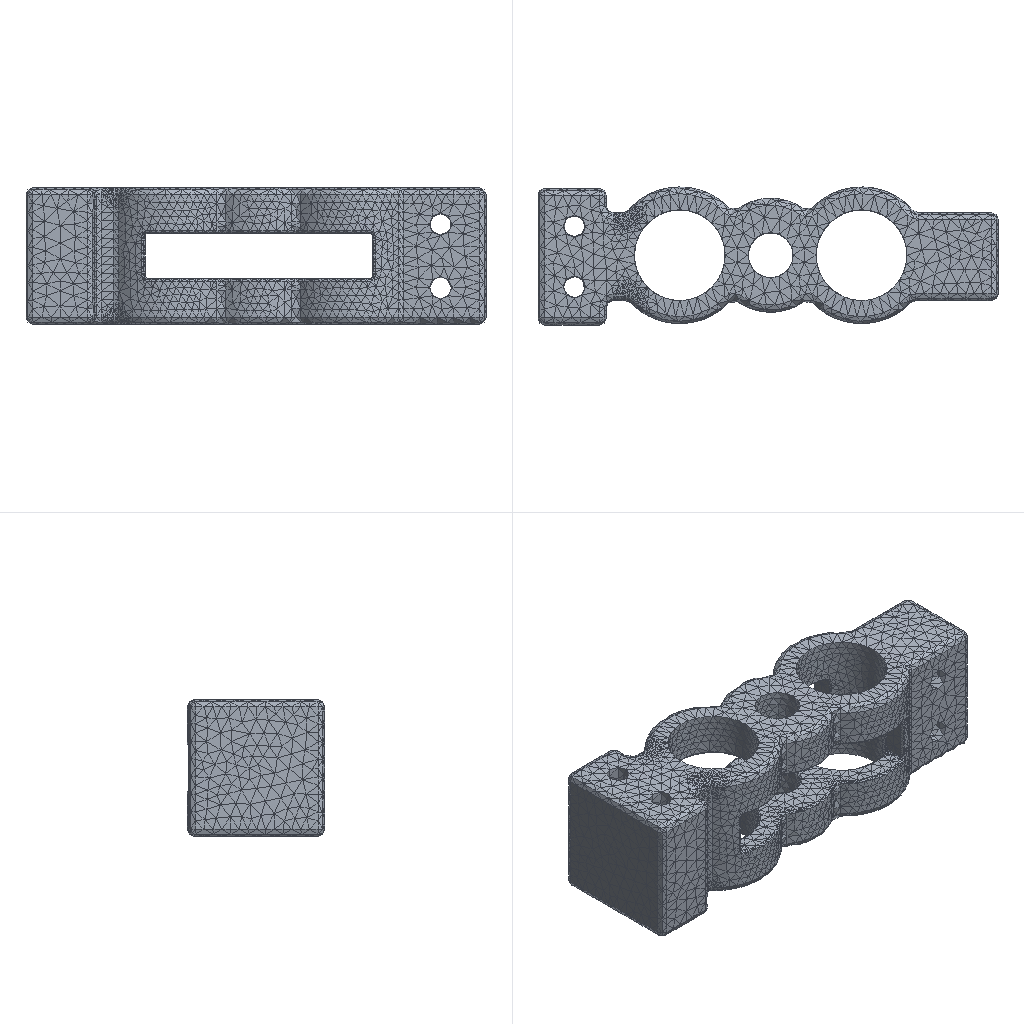Simulation study | ansys workbench
Set-up summary:
category,name,step,type,value,unit,region
solver,ansys_workbench
units,mm-N-s-tonne (MPa),,stated,"/units,MPA"
analysis,LS1,,static
load_step,LS1,LS1,static,nsubst=1; time=1
mesh,nodes,,,59608
mesh,elements,,,36199
element_type,SOLID187,,,35849
element_type,SURF154,,,350
material,Structural Steel,,E,200000,tonne s^-2 mm^-1
material,Structural Steel,,nu,0.3
material,Structural Steel,,density,7.85e-09,tonne mm^-3
material,Structural Steel,,conductivity,60.5,tonne mm s^-3 C^-1
material,Structural Steel,,specific_heat,4.34e+08,mm^2 s^-2 C^-1
material,Structural Steel,,cte,1.2e-05,C^-1
material,Structural Steel,,permeability,10000
material,Structural Steel,,resistivity,0.00017,ohm mm
load,Define Force Using Surface Effect Elements,LS1,surface-effect pres face 2,1.644,,SURF154 #2
bc,Fixed Supports,model,fixed,[dofs=ALL],,_FIXEDSU
named_set,_FIXEDSU,,node,576
Ansys APDL input file, long lists of numbers shortened:
/batch
/config,noeldb,1     ! force off writing results to database
*get,_wallstrt,active,,time,wall
! ANSYS input file written by Workbench version 2025 R2
! File used for geometry attach:
/title,wbnew--____ (A5)
! ****** Begin Custom Load Command Snippet ******
/COM, ACT Extensions:
/COM,     LSDYNA, 2025.2
/COM,/COM,     ANSYSMotion, 2025.2
/COM,
! ****** End   Custom Load Command Snippet ******
*DIM,_wb_ProjectScratch_dir,string,248
_wb_ProjectScratch_dir(1) = ''
*DIM,_wb_SolverFiles_dir,string,248
_wb_SolverFiles_dir(1) = ''
*DIM,_wb_userfiles_dir,string,248
_wb_userfiles_dir(1) = ''
/com,--- Data in consistent NMM units. See Solving Units in the help system for more information.
/units,MPA
/nopr
/wb,file,start              !  signify a WB generated input file
/prep7
! Turn off shape checking because checks already performed inside WB mesher.
! See help system for more information.
SHPP,OFF,,NOWARN
/nolist
etcon,set             ! allow ANSYS to choose best KEYOP's for 180x elements, resets any applicable keyopt to MAPDL defaults
/com,*********** Send User Defined Coordinate System(s) ***********
local,12,0,-71.019,0.4245,29.547,0.,0.,0.
local,13,0,-71.559,18.969,29.548,0.,0.,0.
local,14,0,-71.559,18.969,0.4524,0.,0.,0.
local,15,0,-71.019,0.4245,0.4529,0.,0.,0.
csys,0
/com,*********** Nodes for the whole assembly ***********
nblock,3,,65568
(1i9,3e20.9e3)
        1    -5.000000000E+01     1.000000000E+01     3.000000000E+01
! (59607 more lines like these left out)
-1
/wb,elem,start            !  set before creation of elements
/com,*********** Elements for Body 1 'Solid' ***********
et,1,187
MAT,1 $ TYPE,1 $ REAL,1 $ SECNUM,1 $ ESYS,0
eblock,11,COMPACT,,35849
(11i9)
        1     5950     9015     7975     8565    46217    57922    46214    46215    59404    57920
! (35848 more lines like these left out)
-1
secnum,1    ! reset the section ID to default
/wb,elem,end               !  done creating elements
toffst,273.15,      ! Temperature offset from absolute zero
/com,*********** Set Reference Temperature ***********
tref,22.
/wb,mat,start              !  starting to send materials
/com,*********** Send Materials ***********
Temperature = 'TEMP' ! Temperature
MP,DENS,1,7.85e-09,	! tonne mm^-3
MP,ALPX,1,1.2e-05,	! C^-1
MP,C,1,434000000,	! mm^2 s^-2 C^-1
MP,KXX,1,60.5,	! tonne mm s^-3 C^-1
MP,RSVX,1,0.00017,	! ohm mm
MP,EX,1,200000,	! tonne s^-2 mm^-1
MP,NUXY,1,0.3,
MP,MURX,1,10000,
/wb,mat,end                !  done sending materials
!************************* Model Summary ********************
!Solid,	结构钢,	matid,	1
!************************* End Model Summary ********************
! get the diagonal of the bounding box. Needed later for other things
*get,_xmin,node,,mnloc,x
*get,_ymin,node,,mnloc,y
*get,_zmin,node,,mnloc,z
*get,_xmax,node,,mxloc,x
*get,_ymax,node,,mxloc,y
*get,_zmax,node,,mxloc,z
_ASMDIAG=(_xmax-_xmin)*(_xmax-_xmin)+(_ymax-_ymin)*(_ymax-_ymin)+(_zmax-_zmin)*(_zmax-_zmin)
_ASMDIAG=SQRT(_ASMDIAG)
/wb,contact,start          !  starting to send contact
/wb,contact,end            !  done creating contacts
/golist
/wb,load,start             !  starting to send loads
/com,*********** Fixed Supports ***********
CMBLOCK,_FIXEDSU,NODE,      576
(8i10)
       287      -294       343      -350       514      -521       570      -577
! (71 more lines like these left out)
cmsel,s,_FIXEDSU
d,all,all
nsel,all
/com,*********** Define Force Using Surface Effect Elements ***********
local,16,0,0.,0.,0.,0.,0.,0.
csys,0
et,2,154
MAT,2 $ TYPE,2 $ REAL,2 $ SECNUM,2 $ ESYS,16
eblock,11,COMPACT,,350
(11i9)
    47220      791      790     4586     4586    14511    14513     4586    14519
! (349 more lines like these left out)
-1
secnum,1    ! reset the section ID to default
esel,s,type,,2
keyop,2,2,1         ! Apply load in local coordinate system
keyop,2,7,1         ! Use original area so load is constant in large deformation
esel,all
/gst,on,on
fini
*get,_numnode,node,0,count
*get,_numelem,elem,0,count
*get, _MAXELEMNUM, elem, 0, NUM, MAX
*get, _MAXNODENUM, node, 0, NUM, MAX
*get, _MAXELEMTYPE, etyp, 0, NUM, MAX
*get, _MAXREALCONST, rcon, 0, NUM, MAX
/go
/wb,load,end               !  done creating loads
/com,--- Number of total nodes = %_numnode%
/com,--- Number of contact elements = 350
/com,--- Number of spring elements = 0
/com,--- Number of bearing elements = 0
/com,--- Number of solid elements = 35849
/com,--- Number of condensed parts = 0
/com,--- Number of total elements = %_numelem%
*get,_wallbsol,active,,time,wall
/com,****************************************************************************
/com,*************************    SOLUTION       ********************************
/com,****************************************************************************
/solu
antype,0                   ! static analysis
_thickRatio=  1     ! Ratio of thick parts in the model
eqsl,pcg,1e-8,,,,,,1
cntr,print,1               ! print out contact info and also make no initial contact an error
cncheck,dmp		!	Enable program controlled contact splitting for distributed memory parallel run
dmpoption,emat,no             ! Don't combine emat file for DANSYS
dmpoption,esav,no             ! Don't combine esav file for DANSYS
nldiag,cont,iter           ! print out contact info each equilibrium iteration
rescontrol,,none                 ! Do not keep any restart files
/com,****************************************************
/com,******************* SOLVE FOR LS 1 OF 1 ****************
esel,s,type,,2
nsle
sfe,all,1,pres,1,0.
sfe,all,2,pres,1,1.644
sfe,all,3,pres,1,0.
nsel,all
esel,all
/nopr
/gopr
nsub,1,1,1
time,1.
outres,erase
outres,all,none
outres,nsol,all,
outres,rsol,all
outres,eangl,all
outres,etmp,all
outres,veng,all
outres,strs,all,
outres,epel,all,
outres,eppl,all,
outres,cont,all,
! *********** WB SOLVE COMMAND ***********
! check interactive state
*get,ANSINTER_,active,,int
*if,ANSINTER_,ne,0,then
/eof
*endif
solve
/com *************** Write FE CONNECTORS *********
CEWRITE,file,ce,,INTE
/com,****************************************************
/com,*************** FINISHED SOLVE FOR LS 1 *************
*get,_wallasol,active,,time,wall
/nopr
*get,_numnode,node,0,count
*get,_numelem,elem,0,count
*get, _MAXELEMNUM, elem, 0, NUM, MAX
*get, _MAXNODENUM, node, 0, NUM, MAX,,,INTERNAL
*get, _MAXELEMTYPE, etyp, 0, NUM, MAX
*get, _MAXREALCONST, rcon, 0, NUM, MAX
*get,_NSOLTHREADS,active,0,ntfs
*get,_NSOLPROCESSES,active,0,npfs
/gopr
*get,_PCGITER,active,,solu,cgiter
/post1
xmlo,ENCODING,ISO-8859-1
xmlo,parm
/xml,parm,xml
fini
/gopr
*get,_walldone,active,,time,wall
_preptime=(_wallbsol-_wallstrt)*3600
_solvtime=(_wallasol-_wallbsol)*3600
_posttime=(_walldone-_wallasol)*3600
_totaltim=(_walldone-_wallstrt)*3600
*get,_dlbratio,active,0,solu,dlbr
*get,_combtime,active,0,solu,comb
*get,_ssmode,active,0,solu,ssmm
*get,_ndofs,active,0,solu,ndof
*get,_sol_end_time,active,0,set,time
*if,_sol_end_time,eq,1.,then
/fclean				!clean distributed files
*endif
/com,--- Total number of nodes = %_numnode%
/com,--- Total number of elements = %_numelem%
/com,--- Element load balance ratio = %_dlbratio%
/com,--- Time to combine distributed files = %_combtime%
/com,--- Sparse memory mode = %_ssmode%
/com,--- Number of DOF = %_ndofs%
/wb,file,end               ! done with WB generated input
Results summary:
result,analyses[0].index,,,1
result,analyses[0].system,,,SYS
result,analyses[0].deck,,,deck.dat
result,analyses[0].solve_status,,,completed
result,analyses[0].analysis_type,,,static
result,analyses[0].physics,,,mechanical
result,analyses[0].unit_system,,,"NMM: mm, ton, N, s, mV, mA, degC"
result,analyses[0].n_sets,,,1
result,analyses[0].load_steps[0].set,set=1,,1
result,analyses[0].load_steps[0].time_or_freq,set=1,,1
result,analyses[0].load_steps[0].max_displacement_magnitude,set=1,,0.1192
result,analyses[0].load_steps[0].max_von_mises_nodal,set=1,,207.59
result,analyses[0].load_steps[0].reaction_force_sum_xyz[1],set=1,,-1.76905e-06
result,analyses[0].load_steps[0].reaction_force_sum_xyz[2],set=1,,-999.891
result,analyses[0].load_steps[0].reaction_force_sum_xyz[3],set=1,,-1.89222e-07
result,geometry_export[0][0],,,.step
result,geometry_export[0][1],,,ok
result,geometry_export[0][2],,,1